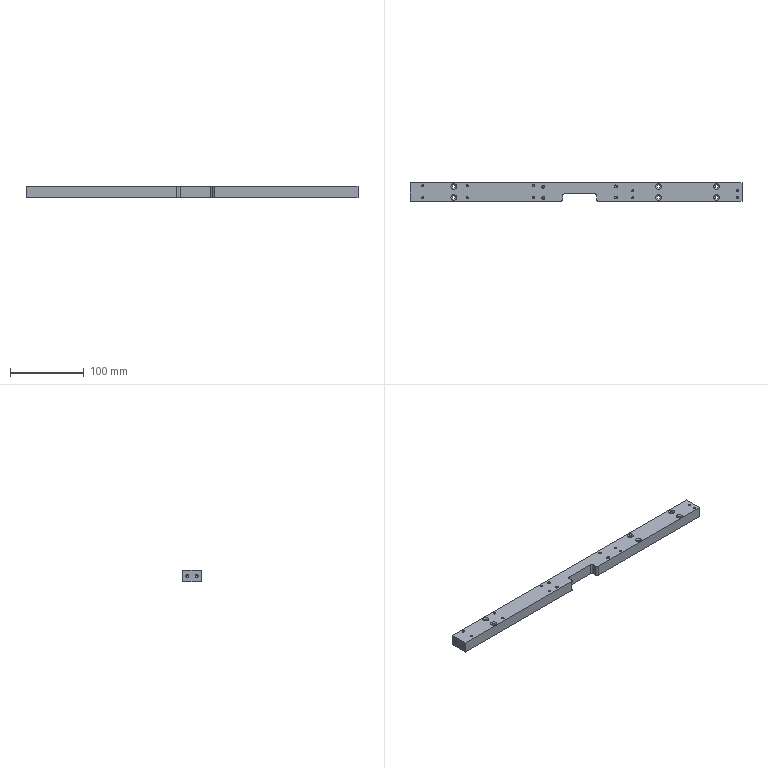Part | STEP file | Chassis spacer strip | 1 solid | 86 faces | box 450 x 25 x 15 mm | volume 159345 mm3 | cone 48 | cylinder 28 | plane 10 | commonest cylinder face diameters 2.5 x10 3.3 x8 4.5 x6 5 x4